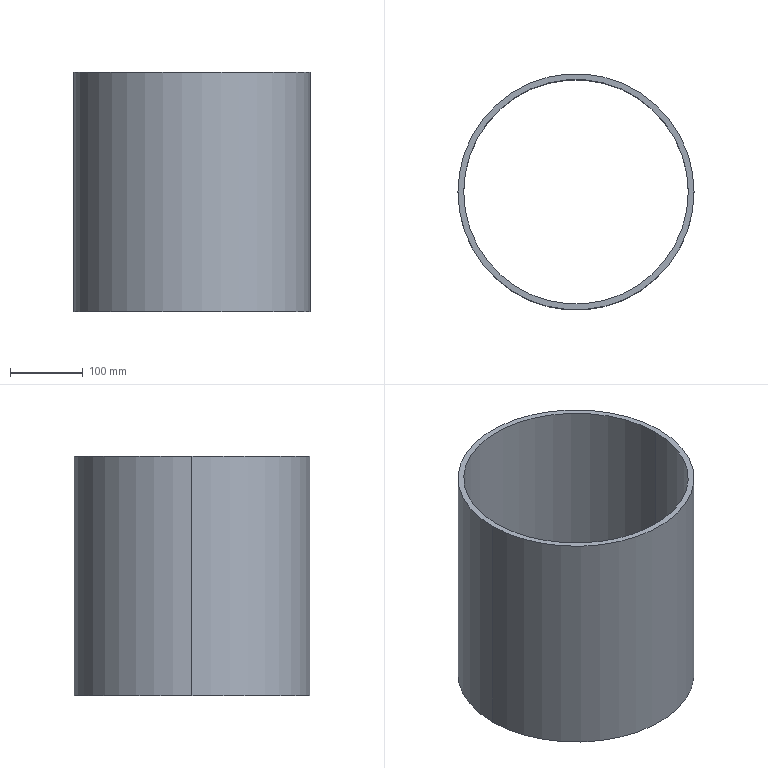Part | SolidWorks | features Extrusion 1 | 1 solid | 6 faces | box 325 x 325 x 330 mm | volume 2629136 mm3 | cylinder 4 | plane 2 | commonest cylinder face diameters 309 x2 325 x2
STEP:
#1=CARTESIAN_POINT('',(-154.5,0.,330.));
#2=VERTEX_POINT('',#1);
#3=CARTESIAN_POINT('',(154.5,0.,330.));
#4=VERTEX_POINT('',#3);
#5=CARTESIAN_POINT('',(0.,0.,330.));
#6=DIRECTION('',(0.,0.,1.));
#7=DIRECTION('',(1.,0.,0.));
#8=AXIS2_PLACEMENT_3D('',#5,#6,#7);
#9=CIRCLE('',#8,154.5);
#10=EDGE_CURVE('',#2,#4,#9,.T.);
#11=ORIENTED_EDGE('',*,*,#10,.T.);
#12=CARTESIAN_POINT('',(154.5,0.,0.));
#13=VERTEX_POINT('',#12);
#14=CARTESIAN_POINT('',(154.5,0.,330.));
#15=DIRECTION('',(0.,0.,-1.));
#16=VECTOR('',#15,1000.);
#17=LINE('',#14,#16);
#18=EDGE_CURVE('',#4,#13,#17,.T.);
#19=ORIENTED_EDGE('',*,*,#18,.T.);
#20=CARTESIAN_POINT('',(-154.5,0.,0.));
#21=VERTEX_POINT('',#20);
#22=CARTESIAN_POINT('',(0.,0.,0.));
#23=DIRECTION('',(0.,0.,1.));
#24=DIRECTION('',(1.,0.,0.));
#25=AXIS2_PLACEMENT_3D('',#22,#23,#24);
#26=CIRCLE('',#25,154.5);
#27=EDGE_CURVE('',#21,#13,#26,.T.);
#28=ORIENTED_EDGE('',*,*,#27,.F.);
#29=CARTESIAN_POINT('',(-154.5,0.,330.));
#30=DIRECTION('',(0.,0.,-1.));
#31=VECTOR('',#30,1000.);
#32=LINE('',#29,#31);
#33=EDGE_CURVE('',#2,#21,#32,.T.);
#34=ORIENTED_EDGE('',*,*,#33,.F.);
#35=EDGE_LOOP('',(#11,#19,#28,#34));
#36=FACE_OUTER_BOUND('',#35,.T.);
#37=CARTESIAN_POINT('',(0.,0.,330.));
#38=DIRECTION('',(0.,0.,-1.));
#39=DIRECTION('',(-1.,0.,0.));
#40=AXIS2_PLACEMENT_3D('',#37,#38,#39);
#41=CYLINDRICAL_SURFACE('',#40,154.5);
#42=ADVANCED_FACE('',(#36),#41,.F.);
#43=CARTESIAN_POINT('',(162.5,0.,330.));
#44=VERTEX_POINT('',#43);
#45=CARTESIAN_POINT('',(-162.5,0.,330.));
#46=VERTEX_POINT('',#45);
#47=CARTESIAN_POINT('',(0.,0.,330.));
#48=DIRECTION('',(0.,0.,1.));
#49=DIRECTION('',(1.,0.,0.));
#50=AXIS2_PLACEMENT_3D('',#47,#48,#49);
#51=CIRCLE('',#50,162.5);
#52=EDGE_CURVE('',#44,#46,#51,.T.);
#53=ORIENTED_EDGE('',*,*,#52,.F.);
#54=CARTESIAN_POINT('',(162.5,0.,0.));
#55=VERTEX_POINT('',#54);
#56=CARTESIAN_POINT('',(162.5,0.,330.));
#57=DIRECTION('',(0.,0.,-1.));
#58=VECTOR('',#57,1000.);
#59=LINE('',#56,#58);
#60=EDGE_CURVE('',#44,#55,#59,.T.);
#61=ORIENTED_EDGE('',*,*,#60,.T.);
#62=CARTESIAN_POINT('',(-162.5,0.,0.));
#63=VERTEX_POINT('',#62);
#64=CARTESIAN_POINT('',(0.,0.,0.));
#65=DIRECTION('',(0.,0.,1.));
#66=DIRECTION('',(1.,0.,0.));
#67=AXIS2_PLACEMENT_3D('',#64,#65,#66);
#68=CIRCLE('',#67,162.5);
#69=EDGE_CURVE('',#55,#63,#68,.T.);
#70=ORIENTED_EDGE('',*,*,#69,.T.);
#71=CARTESIAN_POINT('',(-162.5,0.,330.));
#72=DIRECTION('',(0.,0.,-1.));
#73=VECTOR('',#72,1000.);
#74=LINE('',#71,#73);
#75=EDGE_CURVE('',#46,#63,#74,.T.);
#76=ORIENTED_EDGE('',*,*,#75,.F.);
#77=EDGE_LOOP('',(#53,#61,#70,#76));
#78=FACE_OUTER_BOUND('',#77,.T.);
#79=CARTESIAN_POINT('',(0.,0.,330.));
#80=DIRECTION('',(0.,0.,-1.));
#81=DIRECTION('',(-1.,0.,0.));
#82=AXIS2_PLACEMENT_3D('',#79,#80,#81);
#83=CYLINDRICAL_SURFACE('',#82,162.5);
#84=ADVANCED_FACE('',(#78),#83,.T.);
#85=CARTESIAN_POINT('',(0.,0.,330.));
#86=DIRECTION('',(0.,0.,1.));
#87=DIRECTION('',(1.,0.,0.));
#88=AXIS2_PLACEMENT_3D('',#85,#86,#87);
#89=CIRCLE('',#88,162.5);
#90=EDGE_CURVE('',#46,#44,#89,.T.);
#91=ORIENTED_EDGE('',*,*,#90,.T.);
#92=ORIENTED_EDGE('',*,*,#52,.T.);
#93=EDGE_LOOP('',(#91,#92));
#94=FACE_OUTER_BOUND('',#93,.T.);
#95=ORIENTED_EDGE('',*,*,#10,.F.);
#96=CARTESIAN_POINT('',(0.,0.,330.));
#97=DIRECTION('',(0.,0.,1.));
#98=DIRECTION('',(1.,0.,0.));
#99=AXIS2_PLACEMENT_3D('',#96,#97,#98);
#100=CIRCLE('',#99,154.5);
#101=EDGE_CURVE('',#4,#2,#100,.T.);
#102=ORIENTED_EDGE('',*,*,#101,.F.);
#103=EDGE_LOOP('',(#95,#102));
#104=FACE_BOUND('',#103,.T.);
#105=CARTESIAN_POINT('',(0.,0.,330.));
#106=DIRECTION('',(0.,0.,1.));
#107=DIRECTION('',(1.,0.,0.));
#108=AXIS2_PLACEMENT_3D('',#105,#106,#107);
#109=PLANE('',#108);
#110=ADVANCED_FACE('',(#94,#104),#109,.T.);
#111=CARTESIAN_POINT('',(0.,0.,0.));
#112=DIRECTION('',(0.,0.,1.));
#113=DIRECTION('',(1.,0.,0.));
#114=AXIS2_PLACEMENT_3D('',#111,#112,#113);
#115=CIRCLE('',#114,162.5);
#116=EDGE_CURVE('',#63,#55,#115,.T.);
#117=ORIENTED_EDGE('',*,*,#116,.F.);
#118=ORIENTED_EDGE('',*,*,#69,.F.);
#119=EDGE_LOOP('',(#117,#118));
#120=FACE_OUTER_BOUND('',#119,.T.);
#121=ORIENTED_EDGE('',*,*,#27,.T.);
#122=CARTESIAN_POINT('',(0.,0.,0.));
#123=DIRECTION('',(0.,0.,1.));
#124=DIRECTION('',(1.,0.,0.));
#125=AXIS2_PLACEMENT_3D('',#122,#123,#124);
#126=CIRCLE('',#125,154.5);
#127=EDGE_CURVE('',#13,#21,#126,.T.);
#128=ORIENTED_EDGE('',*,*,#127,.T.);
#129=EDGE_LOOP('',(#121,#128));
#130=FACE_BOUND('',#129,.T.);
#131=CARTESIAN_POINT('',(0.,0.,0.));
#132=DIRECTION('',(0.,0.,1.));
#133=DIRECTION('',(1.,0.,0.));
#134=AXIS2_PLACEMENT_3D('',#131,#132,#133);
#135=PLANE('',#134);
#136=ADVANCED_FACE('',(#120,#130),#135,.F.);
#137=ORIENTED_EDGE('',*,*,#60,.F.);
#138=ORIENTED_EDGE('',*,*,#90,.F.);
#139=ORIENTED_EDGE('',*,*,#75,.T.);
#140=ORIENTED_EDGE('',*,*,#116,.T.);
#141=EDGE_LOOP('',(#137,#138,#139,#140));
#142=FACE_OUTER_BOUND('',#141,.T.);
#143=CARTESIAN_POINT('',(0.,0.,330.));
#144=DIRECTION('',(0.,0.,-1.));
#145=DIRECTION('',(-1.,0.,0.));
#146=AXIS2_PLACEMENT_3D('',#143,#144,#145);
#147=CYLINDRICAL_SURFACE('',#146,162.5);
#148=ADVANCED_FACE('',(#142),#147,.T.);
#149=ORIENTED_EDGE('',*,*,#18,.F.);
#150=ORIENTED_EDGE('',*,*,#101,.T.);
#151=ORIENTED_EDGE('',*,*,#33,.T.);
#152=ORIENTED_EDGE('',*,*,#127,.F.);
#153=EDGE_LOOP('',(#149,#150,#151,#152));
#154=FACE_OUTER_BOUND('',#153,.T.);
#155=CARTESIAN_POINT('',(0.,0.,330.));
#156=DIRECTION('',(0.,0.,-1.));
#157=DIRECTION('',(-1.,0.,0.));
#158=AXIS2_PLACEMENT_3D('',#155,#156,#157);
#159=CYLINDRICAL_SURFACE('',#158,154.5);
#160=ADVANCED_FACE('',(#154),#159,.F.);
#161=CLOSED_SHELL('',(#42,#84,#110,#136,#148,#160));
#162=MANIFOLD_SOLID_BREP('',#161);
#163=CARTESIAN_POINT('',(0.,0.,0.));
#164=DIRECTION('',(0.,0.,1.));
#165=DIRECTION('',(1.,0.,0.));
#166=AXIS2_PLACEMENT_3D('',#163,#164,#165);
#167=(LENGTH_UNIT()NAMED_UNIT(*)SI_UNIT(.MILLI.,.METRE.));
#168=UNCERTAINTY_MEASURE_WITH_UNIT(LENGTH_MEASURE(0.00001),#167,'','');
#169=(NAMED_UNIT(*)PLANE_ANGLE_UNIT()SI_UNIT($,.RADIAN.));
#170=(NAMED_UNIT(*)SI_UNIT($,.STERADIAN.)SOLID_ANGLE_UNIT());
#171=(GEOMETRIC_REPRESENTATION_CONTEXT(3)GLOBAL_UNCERTAINTY_ASSIGNED_CONTEXT((#168))GLOBAL_UNIT_ASSIGNED_CONTEXT((#167,#169,#170))REPRESENTATION_CONTEXT('',''));
#172=ADVANCED_BREP_SHAPE_REPRESENTATION('',(#162,#166),#171);